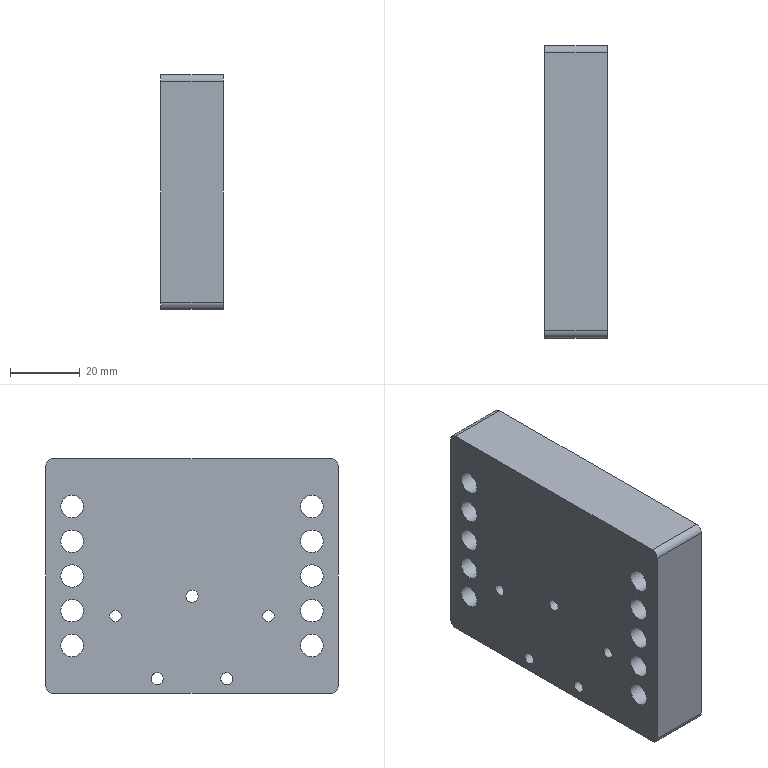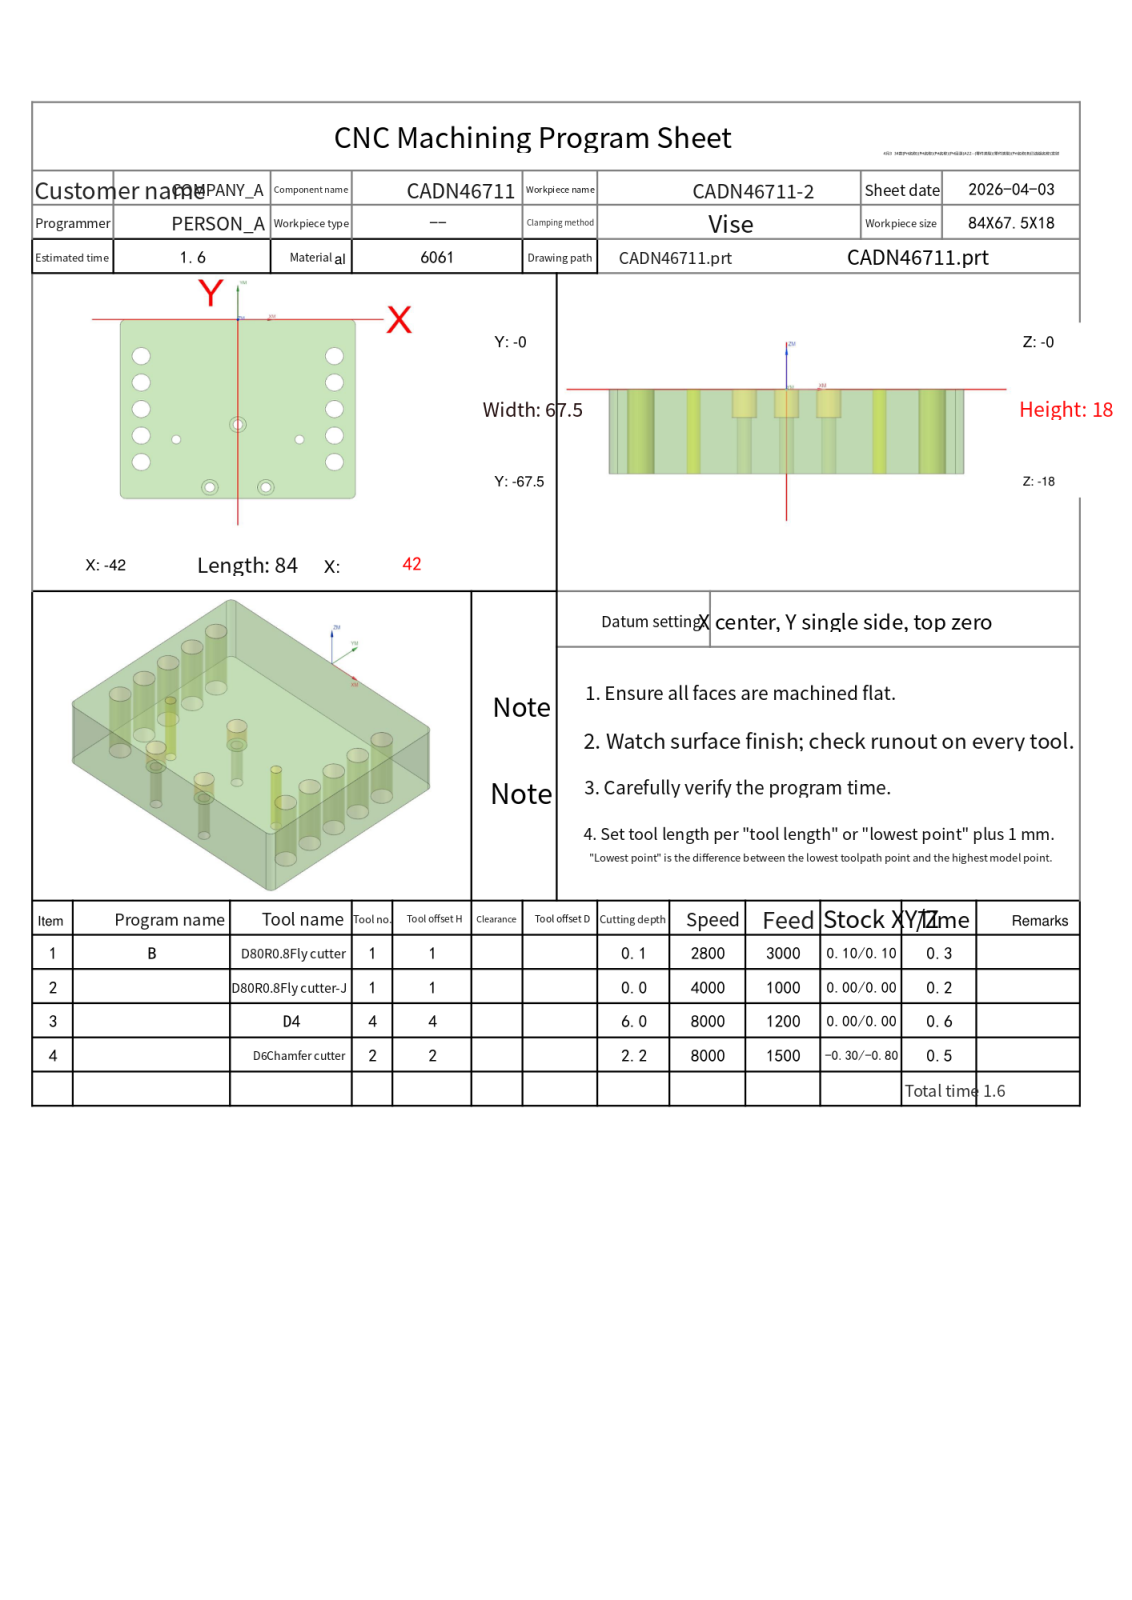NC program | NX | posted by the shop | part box 18 x 84 x 67.5 mm
Whole program:
%
O0001
(Machine time: 2.44 MIN)
(===Total Tool:3===)
(T1=D80R0.8 Fly cutter D=80.  R=0.8  D-  H01 Z=0.    )
(T4=D4      D=4.   R=0.   D-  H04 Z=-6.   )
(T2=D6 Chamfer cutter   D=6.   R=0.   D-  H02 Z=-2.2  )
G80 G90 G17 G49 G40
G91 G28 Z0
M01
N1 T01 M06
(D80R0.8 Fly cutter  D=80. R=0.8 H=01 ce=0.10 di=0.10)
G00 G90 G54 X94.097 Y-31.803 M03 S2800
G43 H01 Z20.
M08
Z3.525
G01 Z1.525 F3000.
X82.097 Y-32.052
X-82.097 Y-35.448
X-94.097 Y-35.697
Z3.525
G00 X94.097 Y-31.803
Z3.05
G01 Z1.05
X82.097 Y-32.052
X-82.097 Y-35.448
X-94.097 Y-35.697
Z3.05
G00 X94.097 Y-31.803
Z2.575
G01 Z.575
X82.097 Y-32.052
X-82.097 Y-35.448
X-94.097 Y-35.697
Z2.575
G00 X94.097 Y-31.803
Z2.1
G01 Z.1
X82.097 Y-32.052
X-82.097 Y-35.448
X-94.097 Y-35.697
Z2.1
G00 Z20.
G91 G28 Z0.0
M05
M09
G91 G28 Z0.0
M01
N2 T01 M06
(D80R0.8 Fly cutter-J  D=80. R=0.8 H=01 ce=0.00 di=0.00)
G00 G90 G54 X93.999 Y-31.807 M03 S4000
G43 H01 Z20.
M08
Z2.
G01 Z0.0 F1000.
X81.999 Y-32.055
X-81.999 Y-35.445
X-93.999 Y-35.693
Z2.
G00 Z20.
G91 G28 Z0.0
M05
M09
G91 G28 Z0.0
M01
N3 T04 M06
(D4  D=4. R=0. H=04 ce=0.07 di=0.00)
G00 G90 G54 X-10. Y-63.3 M03 S8000
G43 H04 Z20.
M08
Z.3
G03 X-9.535 Y-63.765 I.465 J0.0 F1200.
X-9.07 Y-63.3 I0.0 J.465
X-9.07 Y-63.3 Z.1 I-.93 J0.0
X-9.07 Y-63.3 Z-.1 I-.93 J0.0
X-9.07 Y-63.3 Z-.3 I-.93 J0.0
X-9.07 Y-63.3 Z-.5 I-.93 J0.0
X-9.07 Y-63.3 Z-.7 I-.93 J0.0
X-9.07 Y-63.3 Z-.9 I-.93 J0.0
X-9.07 Y-63.3 Z-1.1 I-.93 J0.0
X-9.07 Y-63.3 Z-1.3 I-.93 J0.0
X-9.07 Y-63.3 Z-1.5 I-.93 J0.0
X-9.07 Y-63.3 Z-1.7 I-.93 J0.0
X-9.07 Y-63.3 Z-1.9 I-.93 J0.0
X-9.07 Y-63.3 Z-2.1 I-.93 J0.0
X-9.07 Y-63.3 Z-2.3 I-.93 J0.0
X-9.07 Y-63.3 Z-2.5 I-.93 J0.0
X-9.07 Y-63.3 Z-2.7 I-.93 J0.0
X-9.07 Y-63.3 Z-2.9 I-.93 J0.0
X-9.07 Y-63.3 Z-3.1 I-.93 J0.0
X-9.07 Y-63.3 Z-3.3 I-.93 J0.0
X-9.07 Y-63.3 Z-3.5 I-.93 J0.0
X-9.07 Y-63.3 Z-3.7 I-.93 J0.0
X-9.07 Y-63.3 Z-3.9 I-.93 J0.0
X-9.07 Y-63.3 Z-4.1 I-.93 J0.0
X-9.07 Y-63.3 Z-4.3 I-.93 J0.0
X-9.07 Y-63.3 Z-4.5 I-.93 J0.0
X-9.07 Y-63.3 Z-4.7 I-.93 J0.0
X-9.07 Y-63.3 Z-4.9 I-.93 J0.0
X-9.07 Y-63.3 Z-5.1 I-.93 J0.0
X-9.07 Y-63.3 Z-5.3 I-.93 J0.0
X-9.07 Y-63.3 Z-5.5 I-.93 J0.0
X-9.07 Y-63.3 Z-5.7 I-.93 J0.0
X-9.07 Y-63.3 Z-5.9 I-.93 J0.0
X-10.93 Y-63.3 Z-6. I-.93 J0.0
X-10. Y-64.23 I.93 J0.0
X-9.07 Y-63.3 I0.0 J.93
X-10. Y-62.37 I-.93 J0.0
X-10.93 Y-63.3 I0.0 J-.93
X-10.465 Y-63.765 I.465 J0.0
X-10. Y-63.3 I0.0 J.465
G00 Z20.
X10.
Z.3
G03 X10.465 Y-63.765 I.465 J0.0
X10.93 Y-63.3 I0.0 J.465
X10.93 Y-63.3 Z.1 I-.93 J0.0
X10.93 Y-63.3 Z-.1 I-.93 J0.0
X10.93 Y-63.3 Z-.3 I-.93 J0.0
X10.93 Y-63.3 Z-.5 I-.93 J0.0
X10.93 Y-63.3 Z-.7 I-.93 J0.0
X10.93 Y-63.3 Z-.9 I-.93 J0.0
X10.93 Y-63.3 Z-1.1 I-.93 J0.0
X10.93 Y-63.3 Z-1.3 I-.93 J0.0
X10.93 Y-63.3 Z-1.5 I-.93 J0.0
X10.93 Y-63.3 Z-1.7 I-.93 J0.0
X10.93 Y-63.3 Z-1.9 I-.93 J0.0
X10.93 Y-63.3 Z-2.1 I-.93 J0.0
X10.93 Y-63.3 Z-2.3 I-.93 J0.0
X10.93 Y-63.3 Z-2.5 I-.93 J0.0
X10.93 Y-63.3 Z-2.7 I-.93 J0.0
X10.93 Y-63.3 Z-2.9 I-.93 J0.0
X10.93 Y-63.3 Z-3.1 I-.93 J0.0
X10.93 Y-63.3 Z-3.3 I-.93 J0.0
X10.93 Y-63.3 Z-3.5 I-.93 J0.0
X10.93 Y-63.3 Z-3.7 I-.93 J0.0
X10.93 Y-63.3 Z-3.9 I-.93 J0.0
X10.93 Y-63.3 Z-4.1 I-.93 J0.0
X10.93 Y-63.3 Z-4.3 I-.93 J0.0
X10.93 Y-63.3 Z-4.5 I-.93 J0.0
X10.93 Y-63.3 Z-4.7 I-.93 J0.0
X10.93 Y-63.3 Z-4.9 I-.93 J0.0
X10.93 Y-63.3 Z-5.1 I-.93 J0.0
X10.93 Y-63.3 Z-5.3 I-.93 J0.0
X10.93 Y-63.3 Z-5.5 I-.93 J0.0
X10.93 Y-63.3 Z-5.7 I-.93 J0.0
X10.93 Y-63.3 Z-5.9 I-.93 J0.0
X9.07 Y-63.3 Z-6. I-.93 J0.0
X10. Y-64.23 I.93 J0.0
X10.93 Y-63.3 I0.0 J.93
X10. Y-62.37 I-.93 J0.0
X9.07 Y-63.3 I0.0 J-.93
X9.535 Y-63.765 I.465 J0.0
X10. Y-63.3 I0.0 J.465
G00 Z20.
X0.0 Y-39.6
Z.3
G03 X.465 Y-40.065 I.465 J0.0
X.93 Y-39.6 I0.0 J.465
X.93 Y-39.6 Z.1 I-.93 J0.0
X.93 Y-39.6 Z-.1 I-.93 J0.0
X.93 Y-39.6 Z-.3 I-.93 J0.0
X.93 Y-39.6 Z-.5 I-.93 J0.0
X.93 Y-39.6 Z-.7 I-.93 J0.0
X.93 Y-39.6 Z-.9 I-.93 J0.0
X.93 Y-39.6 Z-1.1 I-.93 J0.0
X.93 Y-39.6 Z-1.3 I-.93 J0.0
X.93 Y-39.6 Z-1.5 I-.93 J0.0
X.93 Y-39.6 Z-1.7 I-.93 J0.0
X.93 Y-39.6 Z-1.9 I-.93 J0.0
X.93 Y-39.6 Z-2.1 I-.93 J0.0
X.93 Y-39.6 Z-2.3 I-.93 J0.0
X.93 Y-39.6 Z-2.5 I-.93 J0.0
X.93 Y-39.6 Z-2.7 I-.93 J0.0
X.93 Y-39.6 Z-2.9 I-.93 J0.0
X.93 Y-39.6 Z-3.1 I-.93 J0.0
X.93 Y-39.6 Z-3.3 I-.93 J0.0
X.93 Y-39.6 Z-3.5 I-.93 J0.0
X.93 Y-39.6 Z-3.7 I-.93 J0.0
X.93 Y-39.6 Z-3.9 I-.93 J0.0
X.93 Y-39.6 Z-4.1 I-.93 J0.0
X.93 Y-39.6 Z-4.3 I-.93 J0.0
X.93 Y-39.6 Z-4.5 I-.93 J0.0
X.93 Y-39.6 Z-4.7 I-.93 J0.0
X.93 Y-39.6 Z-4.9 I-.93 J0.0
X.93 Y-39.6 Z-5.1 I-.93 J0.0
X.93 Y-39.6 Z-5.3 I-.93 J0.0
X.93 Y-39.6 Z-5.5 I-.93 J0.0
X.93 Y-39.6 Z-5.7 I-.93 J0.0
X.93 Y-39.6 Z-5.9 I-.93 J0.0
X-.93 Y-39.6 Z-6. I-.93 J0.0
X0.0 Y-40.53 I.93 J0.0
X.93 Y-39.6 I0.0 J.93
X0.0 Y-38.67 I-.93 J0.0
X-.93 Y-39.6 I0.0 J-.93
X-.465 Y-40.065 I.465 J0.0
X0.0 Y-39.6 I0.0 J.465
G00 Z20.
G00 G90 X-10. Y-63.3 M03 S8000
Z20.
Z-2.75
G01 X-9.432 Y-63.572 F600.
X-9.302 Y-63.602
G03 X-9. Y-63.3 I0.0 J.302
X-10. Y-62.3 I-1. J0.0
X-11. Y-63.3 I0.0 J-1.
X-10. Y-64.3 I1. J0.0
X-9. Y-63.3 I0.0 J1.
X-9.122 Y-62.821 I-1. J0.0
X-9.387 Y-62.664 I-.265 J-.145
X-9.632 Y-62.789 I0.0 J-.302
G01 X-10. Y-63.3
Z-6. F10000.
X-9.432 Y-63.572 F600.
X-9.302 Y-63.602
G03 X-9. Y-63.3 I0.0 J.302
X-10. Y-62.3 I-1. J0.0
X-11. Y-63.3 I0.0 J-1.
X-10. Y-64.3 I1. J0.0
X-9. Y-63.3 I0.0 J1.
X-9.122 Y-62.821 I-1. J0.0
X-9.387 Y-62.664 I-.265 J-.145
X-9.632 Y-62.789 I0.0 J-.302
G01 X-10. Y-63.3
G00 Z20.
X10.
Z-2.75
G01 X10.568 Y-63.572
X10.698 Y-63.602
G03 X11. Y-63.3 I0.0 J.302
X10. Y-62.3 I-1. J0.0
X9. Y-63.3 I0.0 J-1.
X10. Y-64.3 I1. J0.0
X11. Y-63.3 I0.0 J1.
X10.878 Y-62.821 I-1. J0.0
X10.613 Y-62.664 I-.265 J-.145
X10.368 Y-62.789 I0.0 J-.302
G01 X10. Y-63.3
Z-6. F10000.
X10.568 Y-63.572 F600.
X10.698 Y-63.602
G03 X11. Y-63.3 I0.0 J.302
X10. Y-62.3 I-1. J0.0
X9. Y-63.3 I0.0 J-1.
X10. Y-64.3 I1. J0.0
X11. Y-63.3 I0.0 J1.
X10.878 Y-62.821 I-1. J0.0
X10.613 Y-62.664 I-.265 J-.145
X10.368 Y-62.789 I0.0 J-.302
G01 X10. Y-63.3
G00 Z20.
X0.0 Y-39.6
Z-2.75
G01 X.568 Y-39.872
X.698 Y-39.902
G03 X1. Y-39.6 I0.0 J.302
X0.0 Y-38.6 I-1. J0.0
X-1. Y-39.6 I0.0 J-1.
X0.0 Y-40.6 I1. J0.0
X1. Y-39.6 I0.0 J1.
X.878 Y-39.121 I-1. J0.0
X.613 Y-38.964 I-.265 J-.145
X.368 Y-39.089 I0.0 J-.302
G01 X0.0 Y-39.6
Z-6. F10000.
X.568 Y-39.872 F600.
X.698 Y-39.902
G03 X1. Y-39.6 I0.0 J.302
X0.0 Y-38.6 I-1. J0.0
X-1. Y-39.6 I0.0 J-1.
X0.0 Y-40.6 I1. J0.0
X1. Y-39.6 I0.0 J1.
X.878 Y-39.121 I-1. J0.0
X.613 Y-38.964 I-.265 J-.145
X.368 Y-39.089 I0.0 J-.302
G01 X0.0 Y-39.6
G00 Z20.
G91 G28 Z0.0
M05
M09
G91 G28 Z0.0
M01
N4 T02 M06
(D6 Chamfer cutter  D=6. R=0. H=02 ce=0.00 di=0.00)
G00 G90 G54 X22. Y-45.25 M03 S8000
G43 H02 Z20.
M08
G98 G81 X22. Y-45.25 Z-2.2 R3. F1000.
X-22.
G80
G00 Z20.
G00 G90 X.293 Y-39.534 M03 S8000
Z20.
Z-1.5
G01 Z-2. F600.
X.308 Y-39.406
X.319 Y-39.225
G03 X0.0 Y-38.3 I-1.5 J0.0
X-1.3 Y-39.6 I0.0 J-1.3
X0.0 Y-40.9 I1.3 J0.0
X1.3 Y-39.6 I0.0 J1.3
X0.0 Y-38.3 I-1.3 J0.0
X-.319 Y-39.225 I1.181 J-.925
G01 X-.308 Y-39.406
X-.293 Y-39.534
Z-1.5
G00 Z20.
X-9.707 Y-63.234
Z-1.5
G01 Z-2.
X-9.692 Y-63.106
X-9.681 Y-62.925
G03 X-10. Y-62. I-1.5 J0.0
X-11.3 Y-63.3 I0.0 J-1.3
X-10. Y-64.6 I1.3 J0.0
X-8.7 Y-63.3 I0.0 J1.3
X-10. Y-62. I-1.3 J0.0
X-10.319 Y-62.925 I1.181 J-.925
G01 X-10.308 Y-63.106
X-10.293 Y-63.234
Z-1.5
G00 Z20.
X9.707 Y-63.366
Z-1.5
G01 Z-2.
X9.692 Y-63.494
X9.681 Y-63.675
G03 X10. Y-64.6 I1.5 J0.0
X11.3 Y-63.3 I0.0 J1.3
X10. Y-62. I-1.3 J0.0
X8.7 Y-63.3 I0.0 J-1.3
X10. Y-64.6 I1.3 J0.0
X10.319 Y-63.675 I-1.181 J.925
G01 X10.308 Y-63.494
X10.293 Y-63.366
Z-1.5
G00 Z20.
G00 G90 X-33.445 Y-13.293 M03 S8000
Z20.
Z-.9
G01 Z-1.4 F1200.
X-33. Y-13.1
G03 X-34.5 Y-11.6 I-1.5 J0.0
X-36.65 Y-13.75 I0.0 J-2.15
X-34.5 Y-15.9 I2.15 J0.0
X-32.35 Y-13.75 I0.0 J2.15
X-34.5 Y-11.6 I-2.15 J0.0
X-36. Y-13.1 I0.0 J-1.5
G01 X-35.555 Y-13.293
Z-.9
G00 Z20.
X-33.445 Y-23.293
Z-.9
G01 Z-1.4
X-33. Y-23.1
G03 X-34.5 Y-21.6 I-1.5 J0.0
X-36.65 Y-23.75 I0.0 J-2.15
X-34.5 Y-25.9 I2.15 J0.0
X-32.35 Y-23.75 I0.0 J2.15
X-34.5 Y-21.6 I-2.15 J0.0
X-36. Y-23.1 I0.0 J-1.5
G01 X-35.555 Y-23.293
Z-.9
G00 Z20.
X-33.445 Y-33.293
Z-.9
G01 Z-1.4
X-33. Y-33.1
G03 X-34.5 Y-31.6 I-1.5 J0.0
X-36.65 Y-33.75 I0.0 J-2.15
X-34.5 Y-35.9 I2.15 J0.0
X-32.35 Y-33.75 I0.0 J2.15
X-34.5 Y-31.6 I-2.15 J0.0
X-36. Y-33.1 I0.0 J-1.5
G01 X-35.555 Y-33.293
Z-.9
G00 Z20.
X-33.445 Y-43.293
Z-.9
G01 Z-1.4
X-33. Y-43.1
G03 X-34.5 Y-41.6 I-1.5 J0.0
X-36.65 Y-43.75 I0.0 J-2.15
X-34.5 Y-45.9 I2.15 J0.0
X-32.35 Y-43.75 I0.0 J2.15
X-34.5 Y-41.6 I-2.15 J0.0
X-36. Y-43.1 I0.0 J-1.5
G01 X-35.555 Y-43.293
Z-.9
G00 Z20.
X-33.445 Y-53.293
Z-.9
G01 Z-1.4
X-33. Y-53.1
G03 X-34.5 Y-51.6 I-1.5 J0.0
X-36.65 Y-53.75 I0.0 J-2.15
X-34.5 Y-55.9 I2.15 J0.0
X-32.35 Y-53.75 I0.0 J2.15
X-34.5 Y-51.6 I-2.15 J0.0
X-36. Y-53.1 I0.0 J-1.5
G01 X-35.555 Y-53.293
Z-.9
G00 Z20.
X35.555
Z-.9
G01 Z-1.4
X36. Y-53.1
G03 X34.5 Y-51.6 I-1.5 J0.0
X32.35 Y-53.75 I0.0 J-2.15
X34.5 Y-55.9 I2.15 J0.0
X36.65 Y-53.75 I0.0 J2.15
X34.5 Y-51.6 I-2.15 J0.0
X33. Y-53.1 I0.0 J-1.5
G01 X33.445 Y-53.293
Z-.9
G00 Z20.
X35.555 Y-43.293
Z-.9
G01 Z-1.4
X36. Y-43.1
G03 X34.5 Y-41.6 I-1.5 J0.0
X32.35 Y-43.75 I0.0 J-2.15
X34.5 Y-45.9 I2.15 J0.0
X36.65 Y-43.75 I0.0 J2.15
X34.5 Y-41.6 I-2.15 J0.0
X33. Y-43.1 I0.0 J-1.5
G01 X33.445 Y-43.293
Z-.9
G00 Z20.
X35.555 Y-33.293
Z-.9
G01 Z-1.4
X36. Y-33.1
G03 X34.5 Y-31.6 I-1.5 J0.0
X32.35 Y-33.75 I0.0 J-2.15
X34.5 Y-35.9 I2.15 J0.0
X36.65 Y-33.75 I0.0 J2.15
X34.5 Y-31.6 I-2.15 J0.0
X33. Y-33.1 I0.0 J-1.5
G01 X33.445 Y-33.293
Z-.9
G00 Z20.
X35.555 Y-23.293
Z-.9
G01 Z-1.4
X36. Y-23.1
G03 X34.5 Y-21.6 I-1.5 J0.0
X32.35 Y-23.75 I0.0 J-2.15
X34.5 Y-25.9 I2.15 J0.0
X36.65 Y-23.75 I0.0 J2.15
X34.5 Y-21.6 I-2.15 J0.0
X33. Y-23.1 I0.0 J-1.5
G01 X33.445 Y-23.293
Z-.9
G00 Z20.
X35.555 Y-13.293
Z-.9
G01 Z-1.4
X36. Y-13.1
G03 X34.5 Y-11.6 I-1.5 J0.0
X32.35 Y-13.75 I0.0 J-2.15
X34.5 Y-15.9 I2.15 J0.0
X36.65 Y-13.75 I0.0 J2.15
X34.5 Y-11.6 I-2.15 J0.0
X33. Y-13.1 I0.0 J-1.5
G01 X33.445 Y-13.293
Z-.9
G00 Z20.
G00 G90 X-30.384 Y-68.2 M03 S7000
Z20.
Z2.5
G01 X-40. Z-1. F1500.
G02 X-42.7 Y-65.5 I0.0 J2.7
G01 Y-2.
G02 X-40. Y.7 I2.7 J0.0
G01 X40.
G02 X42.7 Y-2. I0.0 J-2.7
G01 Y-65.5
G02 X40. Y-68.2 I-2.7 J0.0
G01 X-40.
G02 X-40.497 Y-68.154 I0.0 J2.7
G01 Z1.5
G00 Z20.
M05
M09
G91 G28 Z0.0
G91 G28 Y0.0
M30
%